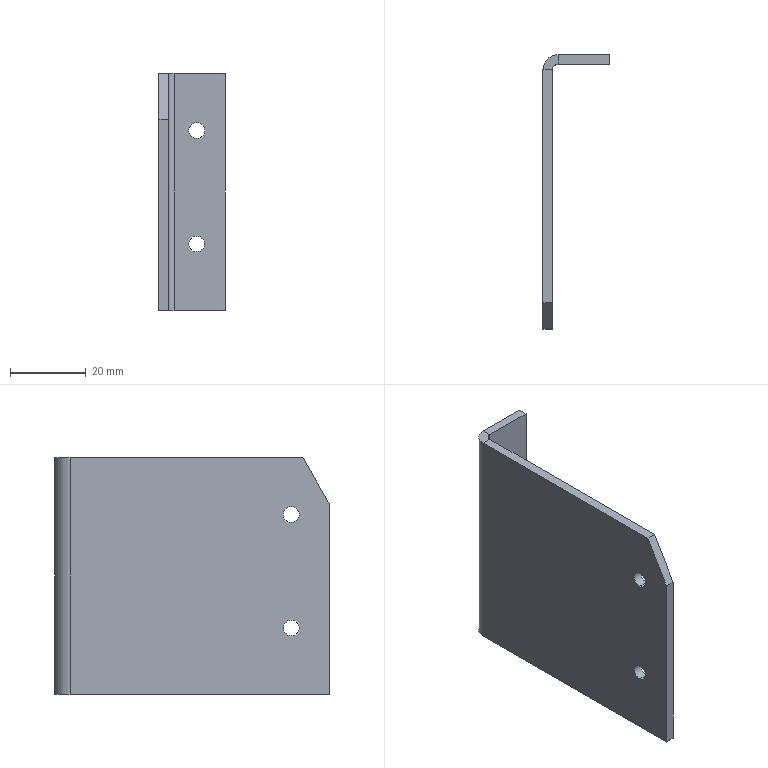Part | STEP file | 64605534 | 1 solid | 23 faces | box 17.5 x 72.5 x 62.5 mm | volume 13245 mm3 | plane 13 | cylinder 10 | commonest cylinder face diameters 4.2 x8 3 x1 8 x1